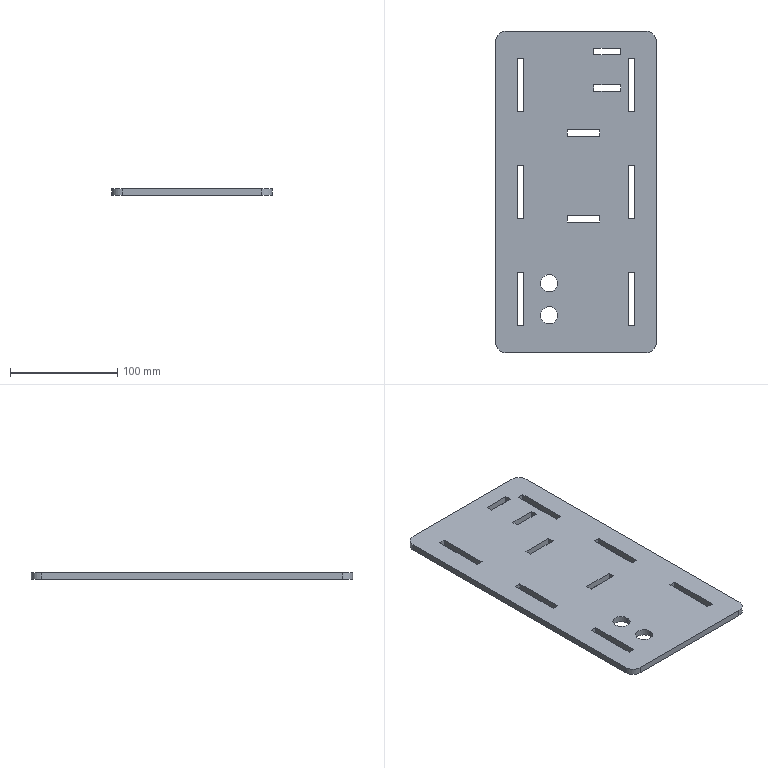Part | SolidWorks | features FlatPattern 1, SMBaseFlange 1, SheetMetal 1 | 1 solid | 54 faces | box 150 x 300 x 6 mm | volume 252312 mm3 | plane 46 | cylinder 8 | commonest cylinder face diameters 16 x4 20 x4